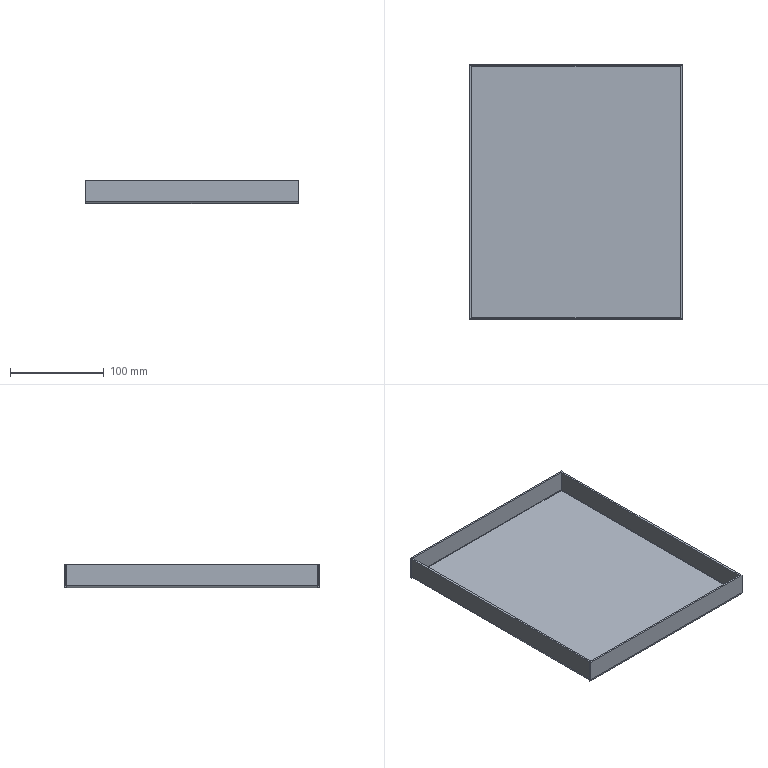Part | STEP file | Rear Base Frame-2 | 1 solid | 34 faces | box 228 x 273 x 25 mm | volume 168843 mm3 | plane 26 | cylinder 8 | commonest cylinder face diameters 1 x4 5 x4
STEP:
#1=CARTESIAN_POINT('',(-827.568,163.879,-2.));
#2=VERTEX_POINT('',#1);
#3=CARTESIAN_POINT('',(-604.568,163.879,-2.));
#4=VERTEX_POINT('',#3);
#5=CARTESIAN_POINT('',(0.,163.879,-2.));
#6=DIRECTION('',(1.,0.,0.));
#7=VECTOR('',#6,1000.);
#8=LINE('',#5,#7);
#9=EDGE_CURVE('',#2,#4,#8,.T.);
#10=ORIENTED_EDGE('',*,*,#9,.T.);
#11=CARTESIAN_POINT('',(-604.568,-104.121,-2.));
#12=VERTEX_POINT('',#11);
#13=CARTESIAN_POINT('',(-604.568,0.,-2.));
#14=DIRECTION('',(0.,-1.,0.));
#15=VECTOR('',#14,1000.);
#16=LINE('',#13,#15);
#17=EDGE_CURVE('',#4,#12,#16,.T.);
#18=ORIENTED_EDGE('',*,*,#17,.T.);
#19=CARTESIAN_POINT('',(-827.568,-104.121,-2.));
#20=VERTEX_POINT('',#19);
#21=CARTESIAN_POINT('',(0.,-104.121,-2.));
#22=DIRECTION('',(-1.,0.,0.));
#23=VECTOR('',#22,1000.);
#24=LINE('',#21,#23);
#25=EDGE_CURVE('',#12,#20,#24,.T.);
#26=ORIENTED_EDGE('',*,*,#25,.T.);
#27=CARTESIAN_POINT('',(-827.568,0.,-2.));
#28=DIRECTION('',(0.,1.,0.));
#29=VECTOR('',#28,1000.);
#30=LINE('',#27,#29);
#31=EDGE_CURVE('',#20,#2,#30,.T.);
#32=ORIENTED_EDGE('',*,*,#31,.T.);
#33=EDGE_LOOP('',(#10,#18,#26,#32));
#34=FACE_OUTER_BOUND('',#33,.T.);
#35=CARTESIAN_POINT('',(0.,0.,-2.));
#36=DIRECTION('',(0.,0.,-1.));
#37=DIRECTION('',(-1.,0.,0.));
#38=AXIS2_PLACEMENT_3D('',#35,#36,#37);
#39=PLANE('',#38);
#40=ADVANCED_FACE('',(#34),#39,.T.);
#41=CARTESIAN_POINT('',(-602.119,-104.121,0.));
#42=VERTEX_POINT('',#41);
#43=CARTESIAN_POINT('',(-602.068,-104.121,0.5));
#44=VERTEX_POINT('',#43);
#45=CARTESIAN_POINT('',(-604.568,-104.121,0.5));
#46=DIRECTION('',(0.,-1.,0.));
#47=DIRECTION('',(0.,0.,1.));
#48=AXIS2_PLACEMENT_3D('',#45,#46,#47);
#49=CIRCLE('',#48,2.5);
#50=EDGE_CURVE('',#42,#44,#49,.T.);
#51=ORIENTED_EDGE('',*,*,#50,.F.);
#52=CARTESIAN_POINT('',(-604.568,-104.121,0.5));
#53=DIRECTION('',(0.,1.,0.));
#54=DIRECTION('',(0.,0.,1.));
#55=AXIS2_PLACEMENT_3D('',#52,#53,#54);
#56=CIRCLE('',#55,2.5);
#57=EDGE_CURVE('',#42,#12,#56,.T.);
#58=ORIENTED_EDGE('',*,*,#57,.T.);
#59=ORIENTED_EDGE('',*,*,#17,.F.);
#60=CARTESIAN_POINT('',(-602.119,163.879,0.));
#61=VERTEX_POINT('',#60);
#62=CARTESIAN_POINT('',(-604.568,163.879,0.5));
#63=DIRECTION('',(0.,-1.,0.));
#64=DIRECTION('',(0.,0.,1.));
#65=AXIS2_PLACEMENT_3D('',#62,#63,#64);
#66=CIRCLE('',#65,2.5);
#67=EDGE_CURVE('',#4,#61,#66,.T.);
#68=ORIENTED_EDGE('',*,*,#67,.T.);
#69=CARTESIAN_POINT('',(-602.068,163.879,0.5));
#70=VERTEX_POINT('',#69);
#71=CARTESIAN_POINT('',(-604.568,163.879,0.5));
#72=DIRECTION('',(0.,-1.,0.));
#73=DIRECTION('',(0.,0.,1.));
#74=AXIS2_PLACEMENT_3D('',#71,#72,#73);
#75=CIRCLE('',#74,2.5);
#76=EDGE_CURVE('',#61,#70,#75,.T.);
#77=ORIENTED_EDGE('',*,*,#76,.T.);
#78=CARTESIAN_POINT('',(-602.068,163.879,0.5));
#79=DIRECTION('',(0.,-1.,0.));
#80=VECTOR('',#79,1000.);
#81=LINE('',#78,#80);
#82=EDGE_CURVE('',#70,#44,#81,.T.);
#83=ORIENTED_EDGE('',*,*,#82,.T.);
#84=EDGE_LOOP('',(#51,#58,#59,#68,#77,#83));
#85=FACE_OUTER_BOUND('',#84,.T.);
#86=CARTESIAN_POINT('',(-604.568,163.879,0.5));
#87=DIRECTION('',(0.,1.,0.));
#88=DIRECTION('',(0.,0.,1.));
#89=AXIS2_PLACEMENT_3D('',#86,#87,#88);
#90=CYLINDRICAL_SURFACE('',#89,2.5);
#91=ADVANCED_FACE('',(#85),#90,.T.);
#92=CARTESIAN_POINT('',(-602.068,163.879,-2.));
#93=VERTEX_POINT('',#92);
#94=CARTESIAN_POINT('',(-830.068,163.879,-2.));
#95=DIRECTION('',(-1.,0.,0.));
#96=VECTOR('',#95,1000.);
#97=LINE('',#94,#96);
#98=EDGE_CURVE('',#93,#4,#97,.T.);
#99=ORIENTED_EDGE('',*,*,#98,.T.);
#100=ORIENTED_EDGE('',*,*,#9,.F.);
#101=CARTESIAN_POINT('',(-830.068,163.879,-2.));
#102=VERTEX_POINT('',#101);
#103=CARTESIAN_POINT('',(-830.068,163.879,-2.));
#104=DIRECTION('',(-1.,0.,0.));
#105=VECTOR('',#104,1000.);
#106=LINE('',#103,#105);
#107=EDGE_CURVE('',#2,#102,#106,.T.);
#108=ORIENTED_EDGE('',*,*,#107,.T.);
#109=CARTESIAN_POINT('',(-830.068,166.379,0.5));
#110=VERTEX_POINT('',#109);
#111=CARTESIAN_POINT('',(-830.068,163.879,0.5));
#112=DIRECTION('',(1.,0.,0.));
#113=DIRECTION('',(0.,0.,1.));
#114=AXIS2_PLACEMENT_3D('',#111,#112,#113);
#115=CIRCLE('',#114,2.5);
#116=EDGE_CURVE('',#102,#110,#115,.T.);
#117=ORIENTED_EDGE('',*,*,#116,.T.);
#118=CARTESIAN_POINT('',(-602.068,166.379,0.5));
#119=VERTEX_POINT('',#118);
#120=CARTESIAN_POINT('',(-830.068,166.379,0.5));
#121=DIRECTION('',(1.,0.,0.));
#122=VECTOR('',#121,1000.);
#123=LINE('',#120,#122);
#124=EDGE_CURVE('',#110,#119,#123,.T.);
#125=ORIENTED_EDGE('',*,*,#124,.T.);
#126=CARTESIAN_POINT('',(-602.068,163.879,0.5));
#127=DIRECTION('',(-1.,0.,0.));
#128=DIRECTION('',(0.,0.,1.));
#129=AXIS2_PLACEMENT_3D('',#126,#127,#128);
#130=CIRCLE('',#129,2.5);
#131=EDGE_CURVE('',#119,#93,#130,.T.);
#132=ORIENTED_EDGE('',*,*,#131,.T.);
#133=EDGE_LOOP('',(#99,#100,#108,#117,#125,#132));
#134=FACE_OUTER_BOUND('',#133,.T.);
#135=CARTESIAN_POINT('',(-830.068,163.879,0.5));
#136=DIRECTION('',(-1.,0.,0.));
#137=DIRECTION('',(0.,0.,1.));
#138=AXIS2_PLACEMENT_3D('',#135,#136,#137);
#139=CYLINDRICAL_SURFACE('',#138,2.5);
#140=ADVANCED_FACE('',(#134),#139,.T.);
#141=CARTESIAN_POINT('',(-830.018,163.879,0.));
#142=VERTEX_POINT('',#141);
#143=CARTESIAN_POINT('',(-830.068,163.879,0.5));
#144=VERTEX_POINT('',#143);
#145=CARTESIAN_POINT('',(-827.568,163.879,0.5));
#146=DIRECTION('',(0.,1.,0.));
#147=DIRECTION('',(0.,0.,-1.));
#148=AXIS2_PLACEMENT_3D('',#145,#146,#147);
#149=CIRCLE('',#148,2.5);
#150=EDGE_CURVE('',#142,#144,#149,.T.);
#151=ORIENTED_EDGE('',*,*,#150,.F.);
#152=CARTESIAN_POINT('',(-827.568,163.879,0.5));
#153=DIRECTION('',(0.,-1.,0.));
#154=DIRECTION('',(0.,0.,-1.));
#155=AXIS2_PLACEMENT_3D('',#152,#153,#154);
#156=CIRCLE('',#155,2.5);
#157=EDGE_CURVE('',#142,#2,#156,.T.);
#158=ORIENTED_EDGE('',*,*,#157,.T.);
#159=ORIENTED_EDGE('',*,*,#31,.F.);
#160=CARTESIAN_POINT('',(-830.018,-104.121,0.));
#161=VERTEX_POINT('',#160);
#162=CARTESIAN_POINT('',(-827.568,-104.121,0.5));
#163=DIRECTION('',(0.,1.,0.));
#164=DIRECTION('',(0.,0.,-1.));
#165=AXIS2_PLACEMENT_3D('',#162,#163,#164);
#166=CIRCLE('',#165,2.5);
#167=EDGE_CURVE('',#20,#161,#166,.T.);
#168=ORIENTED_EDGE('',*,*,#167,.T.);
#169=CARTESIAN_POINT('',(-830.068,-104.121,0.5));
#170=VERTEX_POINT('',#169);
#171=CARTESIAN_POINT('',(-827.568,-104.121,0.5));
#172=DIRECTION('',(0.,1.,0.));
#173=DIRECTION('',(0.,0.,-1.));
#174=AXIS2_PLACEMENT_3D('',#171,#172,#173);
#175=CIRCLE('',#174,2.5);
#176=EDGE_CURVE('',#161,#170,#175,.T.);
#177=ORIENTED_EDGE('',*,*,#176,.T.);
#178=CARTESIAN_POINT('',(-830.068,-104.121,0.5));
#179=DIRECTION('',(0.,1.,0.));
#180=VECTOR('',#179,1000.);
#181=LINE('',#178,#180);
#182=EDGE_CURVE('',#170,#144,#181,.T.);
#183=ORIENTED_EDGE('',*,*,#182,.T.);
#184=EDGE_LOOP('',(#151,#158,#159,#168,#177,#183));
#185=FACE_OUTER_BOUND('',#184,.T.);
#186=CARTESIAN_POINT('',(-827.568,-104.121,0.5));
#187=DIRECTION('',(0.,-1.,0.));
#188=DIRECTION('',(0.,0.,-1.));
#189=AXIS2_PLACEMENT_3D('',#186,#187,#188);
#190=CYLINDRICAL_SURFACE('',#189,2.5);
#191=ADVANCED_FACE('',(#185),#190,.T.);
#192=CARTESIAN_POINT('',(-830.068,-104.121,-2.));
#193=VERTEX_POINT('',#192);
#194=CARTESIAN_POINT('',(-602.068,-104.121,-2.));
#195=DIRECTION('',(1.,0.,0.));
#196=VECTOR('',#195,1000.);
#197=LINE('',#194,#196);
#198=EDGE_CURVE('',#193,#20,#197,.T.);
#199=ORIENTED_EDGE('',*,*,#198,.T.);
#200=ORIENTED_EDGE('',*,*,#25,.F.);
#201=CARTESIAN_POINT('',(-602.068,-104.121,-2.));
#202=VERTEX_POINT('',#201);
#203=CARTESIAN_POINT('',(-602.068,-104.121,-2.));
#204=DIRECTION('',(1.,0.,0.));
#205=VECTOR('',#204,1000.);
#206=LINE('',#203,#205);
#207=EDGE_CURVE('',#12,#202,#206,.T.);
#208=ORIENTED_EDGE('',*,*,#207,.T.);
#209=CARTESIAN_POINT('',(-602.068,-106.621,0.5));
#210=VERTEX_POINT('',#209);
#211=CARTESIAN_POINT('',(-602.068,-104.121,0.5));
#212=DIRECTION('',(-1.,0.,0.));
#213=DIRECTION('',(0.,0.,-1.));
#214=AXIS2_PLACEMENT_3D('',#211,#212,#213);
#215=CIRCLE('',#214,2.5);
#216=EDGE_CURVE('',#202,#210,#215,.T.);
#217=ORIENTED_EDGE('',*,*,#216,.T.);
#218=CARTESIAN_POINT('',(-830.068,-106.621,0.5));
#219=VERTEX_POINT('',#218);
#220=CARTESIAN_POINT('',(-602.068,-106.621,0.5));
#221=DIRECTION('',(-1.,0.,0.));
#222=VECTOR('',#221,1000.);
#223=LINE('',#220,#222);
#224=EDGE_CURVE('',#210,#219,#223,.T.);
#225=ORIENTED_EDGE('',*,*,#224,.T.);
#226=CARTESIAN_POINT('',(-830.068,-104.121,0.5));
#227=DIRECTION('',(1.,0.,0.));
#228=DIRECTION('',(0.,0.,-1.));
#229=AXIS2_PLACEMENT_3D('',#226,#227,#228);
#230=CIRCLE('',#229,2.5);
#231=EDGE_CURVE('',#219,#193,#230,.T.);
#232=ORIENTED_EDGE('',*,*,#231,.T.);
#233=EDGE_LOOP('',(#199,#200,#208,#217,#225,#232));
#234=FACE_OUTER_BOUND('',#233,.T.);
#235=CARTESIAN_POINT('',(-602.068,-104.121,0.5));
#236=DIRECTION('',(1.,0.,0.));
#237=DIRECTION('',(0.,0.,-1.));
#238=AXIS2_PLACEMENT_3D('',#235,#236,#237);
#239=CYLINDRICAL_SURFACE('',#238,2.5);
#240=ADVANCED_FACE('',(#234),#239,.T.);
#241=CARTESIAN_POINT('',(-602.068,-104.121,0.));
#242=VERTEX_POINT('',#241);
#243=CARTESIAN_POINT('',(-602.068,-104.121,0.));
#244=DIRECTION('',(1.,0.,0.));
#245=VECTOR('',#244,1000.);
#246=LINE('',#243,#245);
#247=EDGE_CURVE('',#42,#242,#246,.T.);
#248=ORIENTED_EDGE('',*,*,#247,.T.);
#249=CARTESIAN_POINT('',(-602.068,-104.121,0.));
#250=DIRECTION('',(0.,0.,-1.));
#251=VECTOR('',#250,1000.);
#252=LINE('',#249,#251);
#253=EDGE_CURVE('',#242,#202,#252,.T.);
#254=ORIENTED_EDGE('',*,*,#253,.T.);
#255=ORIENTED_EDGE('',*,*,#207,.F.);
#256=ORIENTED_EDGE('',*,*,#57,.F.);
#257=EDGE_LOOP('',(#248,#254,#255,#256));
#258=FACE_OUTER_BOUND('',#257,.T.);
#259=CARTESIAN_POINT('',(-604.568,-104.121,0.));
#260=DIRECTION('',(0.,1.,0.));
#261=DIRECTION('',(0.,0.,1.));
#262=AXIS2_PLACEMENT_3D('',#259,#260,#261);
#263=PLANE('',#262);
#264=ADVANCED_FACE('',(#258),#263,.T.);
#265=CARTESIAN_POINT('',(-602.068,163.879,23.));
#266=VERTEX_POINT('',#265);
#267=CARTESIAN_POINT('',(-602.068,163.879,0.));
#268=DIRECTION('',(0.,0.,-1.));
#269=VECTOR('',#268,1000.);
#270=LINE('',#267,#269);
#271=EDGE_CURVE('',#266,#70,#270,.T.);
#272=ORIENTED_EDGE('',*,*,#271,.F.);
#273=CARTESIAN_POINT('',(-602.068,-104.121,23.));
#274=VERTEX_POINT('',#273);
#275=CARTESIAN_POINT('',(-602.068,0.,23.));
#276=DIRECTION('',(0.,1.,0.));
#277=VECTOR('',#276,1000.);
#278=LINE('',#275,#277);
#279=EDGE_CURVE('',#274,#266,#278,.T.);
#280=ORIENTED_EDGE('',*,*,#279,.F.);
#281=CARTESIAN_POINT('',(-602.068,-104.121,0.));
#282=DIRECTION('',(0.,0.,1.));
#283=VECTOR('',#282,1000.);
#284=LINE('',#281,#283);
#285=EDGE_CURVE('',#44,#274,#284,.T.);
#286=ORIENTED_EDGE('',*,*,#285,.F.);
#287=ORIENTED_EDGE('',*,*,#82,.F.);
#288=EDGE_LOOP('',(#272,#280,#286,#287));
#289=FACE_OUTER_BOUND('',#288,.T.);
#290=CARTESIAN_POINT('',(-602.068,0.,0.));
#291=DIRECTION('',(-1.,0.,0.));
#292=DIRECTION('',(0.,0.,1.));
#293=AXIS2_PLACEMENT_3D('',#290,#291,#292);
#294=PLANE('',#293);
#295=ADVANCED_FACE('',(#289),#294,.F.);
#296=ORIENTED_EDGE('',*,*,#98,.F.);
#297=CARTESIAN_POINT('',(-602.068,163.879,0.));
#298=VERTEX_POINT('',#297);
#299=CARTESIAN_POINT('',(-602.068,163.879,0.));
#300=DIRECTION('',(0.,0.,1.));
#301=VECTOR('',#300,1000.);
#302=LINE('',#299,#301);
#303=EDGE_CURVE('',#93,#298,#302,.T.);
#304=ORIENTED_EDGE('',*,*,#303,.T.);
#305=CARTESIAN_POINT('',(-830.068,163.879,0.));
#306=DIRECTION('',(-1.,0.,0.));
#307=VECTOR('',#306,1000.);
#308=LINE('',#305,#307);
#309=EDGE_CURVE('',#298,#61,#308,.T.);
#310=ORIENTED_EDGE('',*,*,#309,.T.);
#311=ORIENTED_EDGE('',*,*,#67,.F.);
#312=EDGE_LOOP('',(#296,#304,#310,#311));
#313=FACE_OUTER_BOUND('',#312,.T.);
#314=CARTESIAN_POINT('',(-602.068,163.879,0.));
#315=DIRECTION('',(0.,-1.,0.));
#316=DIRECTION('',(0.,0.,-1.));
#317=AXIS2_PLACEMENT_3D('',#314,#315,#316);
#318=PLANE('',#317);
#319=ADVANCED_FACE('',(#313),#318,.T.);
#320=ORIENTED_EDGE('',*,*,#303,.F.);
#321=ORIENTED_EDGE('',*,*,#131,.F.);
#322=CARTESIAN_POINT('',(-602.068,166.379,23.));
#323=VERTEX_POINT('',#322);
#324=CARTESIAN_POINT('',(-602.068,166.379,0.));
#325=DIRECTION('',(0.,0.,1.));
#326=VECTOR('',#325,1000.);
#327=LINE('',#324,#326);
#328=EDGE_CURVE('',#119,#323,#327,.T.);
#329=ORIENTED_EDGE('',*,*,#328,.T.);
#330=CARTESIAN_POINT('',(-602.068,164.379,23.));
#331=VERTEX_POINT('',#330);
#332=CARTESIAN_POINT('',(-602.068,166.379,23.));
#333=DIRECTION('',(0.,1.,0.));
#334=VECTOR('',#333,1000.);
#335=LINE('',#332,#334);
#336=EDGE_CURVE('',#331,#323,#335,.T.);
#337=ORIENTED_EDGE('',*,*,#336,.F.);
#338=CARTESIAN_POINT('',(-602.068,164.379,0.5));
#339=VERTEX_POINT('',#338);
#340=CARTESIAN_POINT('',(-602.068,164.379,0.));
#341=DIRECTION('',(0.,0.,1.));
#342=VECTOR('',#341,1000.);
#343=LINE('',#340,#342);
#344=EDGE_CURVE('',#339,#331,#343,.T.);
#345=ORIENTED_EDGE('',*,*,#344,.F.);
#346=CARTESIAN_POINT('',(-602.068,163.879,0.5));
#347=DIRECTION('',(-1.,0.,0.));
#348=DIRECTION('',(0.,0.,1.));
#349=AXIS2_PLACEMENT_3D('',#346,#347,#348);
#350=CIRCLE('',#349,0.5);
#351=EDGE_CURVE('',#339,#298,#350,.T.);
#352=ORIENTED_EDGE('',*,*,#351,.T.);
#353=EDGE_LOOP('',(#320,#321,#329,#337,#345,#352));
#354=FACE_OUTER_BOUND('',#353,.T.);
#355=CARTESIAN_POINT('',(-602.068,163.879,0.5));
#356=DIRECTION('',(1.,0.,0.));
#357=DIRECTION('',(0.,0.,-1.));
#358=AXIS2_PLACEMENT_3D('',#355,#356,#357);
#359=PLANE('',#358);
#360=ADVANCED_FACE('',(#354),#359,.T.);
#361=CARTESIAN_POINT('',(-830.068,166.379,23.));
#362=VERTEX_POINT('',#361);
#363=CARTESIAN_POINT('',(-830.068,166.379,0.));
#364=DIRECTION('',(0.,0.,-1.));
#365=VECTOR('',#364,1000.);
#366=LINE('',#363,#365);
#367=EDGE_CURVE('',#362,#110,#366,.T.);
#368=ORIENTED_EDGE('',*,*,#367,.F.);
#369=CARTESIAN_POINT('',(0.,166.379,23.));
#370=DIRECTION('',(-1.,0.,0.));
#371=VECTOR('',#370,1000.);
#372=LINE('',#369,#371);
#373=EDGE_CURVE('',#323,#362,#372,.T.);
#374=ORIENTED_EDGE('',*,*,#373,.F.);
#375=ORIENTED_EDGE('',*,*,#328,.F.);
#376=ORIENTED_EDGE('',*,*,#124,.F.);
#377=EDGE_LOOP('',(#368,#374,#375,#376));
#378=FACE_OUTER_BOUND('',#377,.T.);
#379=CARTESIAN_POINT('',(0.,166.379,0.));
#380=DIRECTION('',(0.,-1.,0.));
#381=DIRECTION('',(0.,0.,-1.));
#382=AXIS2_PLACEMENT_3D('',#379,#380,#381);
#383=PLANE('',#382);
#384=ADVANCED_FACE('',(#378),#383,.F.);
#385=CARTESIAN_POINT('',(-830.068,163.879,0.));
#386=VERTEX_POINT('',#385);
#387=CARTESIAN_POINT('',(-830.068,164.379,0.5));
#388=VERTEX_POINT('',#387);
#389=CARTESIAN_POINT('',(-830.068,163.879,0.5));
#390=DIRECTION('',(1.,0.,0.));
#391=DIRECTION('',(0.,0.,1.));
#392=AXIS2_PLACEMENT_3D('',#389,#390,#391);
#393=CIRCLE('',#392,0.5);
#394=EDGE_CURVE('',#386,#388,#393,.T.);
#395=ORIENTED_EDGE('',*,*,#394,.T.);
#396=CARTESIAN_POINT('',(-830.068,164.379,23.));
#397=VERTEX_POINT('',#396);
#398=CARTESIAN_POINT('',(-830.068,164.379,23.));
#399=DIRECTION('',(0.,0.,-1.));
#400=VECTOR('',#399,1000.);
#401=LINE('',#398,#400);
#402=EDGE_CURVE('',#397,#388,#401,.T.);
#403=ORIENTED_EDGE('',*,*,#402,.F.);
#404=CARTESIAN_POINT('',(-830.068,166.379,23.));
#405=DIRECTION('',(0.,-1.,0.));
#406=VECTOR('',#405,1000.);
#407=LINE('',#404,#406);
#408=EDGE_CURVE('',#362,#397,#407,.T.);
#409=ORIENTED_EDGE('',*,*,#408,.F.);
#410=ORIENTED_EDGE('',*,*,#367,.T.);
#411=ORIENTED_EDGE('',*,*,#116,.F.);
#412=CARTESIAN_POINT('',(-830.068,163.879,0.5));
#413=DIRECTION('',(0.,0.,-1.));
#414=VECTOR('',#413,1000.);
#415=LINE('',#412,#414);
#416=EDGE_CURVE('',#386,#102,#415,.T.);
#417=ORIENTED_EDGE('',*,*,#416,.F.);
#418=EDGE_LOOP('',(#395,#403,#409,#410,#411,#417));
#419=FACE_OUTER_BOUND('',#418,.T.);
#420=CARTESIAN_POINT('',(-830.068,163.879,0.5));
#421=DIRECTION('',(1.,0.,0.));
#422=DIRECTION('',(0.,0.,-1.));
#423=AXIS2_PLACEMENT_3D('',#420,#421,#422);
#424=PLANE('',#423);
#425=ADVANCED_FACE('',(#419),#424,.F.);
#426=CARTESIAN_POINT('',(-830.068,163.879,0.));
#427=DIRECTION('',(-1.,0.,0.));
#428=VECTOR('',#427,1000.);
#429=LINE('',#426,#428);
#430=EDGE_CURVE('',#142,#386,#429,.T.);
#431=ORIENTED_EDGE('',*,*,#430,.T.);
#432=ORIENTED_EDGE('',*,*,#416,.T.);
#433=ORIENTED_EDGE('',*,*,#107,.F.);
#434=ORIENTED_EDGE('',*,*,#157,.F.);
#435=EDGE_LOOP('',(#431,#432,#433,#434));
#436=FACE_OUTER_BOUND('',#435,.T.);
#437=CARTESIAN_POINT('',(-827.568,163.879,0.));
#438=DIRECTION('',(0.,-1.,0.));
#439=DIRECTION('',(0.,0.,-1.));
#440=AXIS2_PLACEMENT_3D('',#437,#438,#439);
#441=PLANE('',#440);
#442=ADVANCED_FACE('',(#436),#441,.T.);
#443=CARTESIAN_POINT('',(-830.068,-104.121,23.));
#444=VERTEX_POINT('',#443);
#445=CARTESIAN_POINT('',(-830.068,-104.121,0.));
#446=DIRECTION('',(0.,0.,-1.));
#447=VECTOR('',#446,1000.);
#448=LINE('',#445,#447);
#449=EDGE_CURVE('',#444,#170,#448,.T.);
#450=ORIENTED_EDGE('',*,*,#449,.F.);
#451=CARTESIAN_POINT('',(-830.068,163.879,23.));
#452=VERTEX_POINT('',#451);
#453=CARTESIAN_POINT('',(-830.068,0.,23.));
#454=DIRECTION('',(0.,-1.,0.));
#455=VECTOR('',#454,1000.);
#456=LINE('',#453,#455);
#457=EDGE_CURVE('',#452,#444,#456,.T.);
#458=ORIENTED_EDGE('',*,*,#457,.F.);
#459=CARTESIAN_POINT('',(-830.068,163.879,0.));
#460=DIRECTION('',(0.,0.,1.));
#461=VECTOR('',#460,1000.);
#462=LINE('',#459,#461);
#463=EDGE_CURVE('',#144,#452,#462,.T.);
#464=ORIENTED_EDGE('',*,*,#463,.F.);
#465=ORIENTED_EDGE('',*,*,#182,.F.);
#466=EDGE_LOOP('',(#450,#458,#464,#465));
#467=FACE_OUTER_BOUND('',#466,.T.);
#468=CARTESIAN_POINT('',(-830.068,0.,0.));
#469=DIRECTION('',(1.,0.,0.));
#470=DIRECTION('',(0.,0.,-1.));
#471=AXIS2_PLACEMENT_3D('',#468,#469,#470);
#472=PLANE('',#471);
#473=ADVANCED_FACE('',(#467),#472,.F.);
#474=ORIENTED_EDGE('',*,*,#198,.F.);
#475=CARTESIAN_POINT('',(-830.068,-104.121,0.));
#476=VERTEX_POINT('',#475);
#477=CARTESIAN_POINT('',(-830.068,-104.121,0.));
#478=DIRECTION('',(0.,0.,1.));
#479=VECTOR('',#478,1000.);
#480=LINE('',#477,#479);
#481=EDGE_CURVE('',#193,#476,#480,.T.);
#482=ORIENTED_EDGE('',*,*,#481,.T.);
#483=CARTESIAN_POINT('',(-602.068,-104.121,0.));
#484=DIRECTION('',(1.,0.,0.));
#485=VECTOR('',#484,1000.);
#486=LINE('',#483,#485);
#487=EDGE_CURVE('',#476,#161,#486,.T.);
#488=ORIENTED_EDGE('',*,*,#487,.T.);
#489=ORIENTED_EDGE('',*,*,#167,.F.);
#490=EDGE_LOOP('',(#474,#482,#488,#489));
#491=FACE_OUTER_BOUND('',#490,.T.);
#492=CARTESIAN_POINT('',(-830.068,-104.121,0.));
#493=DIRECTION('',(0.,1.,0.));
#494=DIRECTION('',(-1.,0.,0.));
#495=AXIS2_PLACEMENT_3D('',#492,#493,#494);
#496=PLANE('',#495);
#497=ADVANCED_FACE('',(#491),#496,.T.);
#498=ORIENTED_EDGE('',*,*,#481,.F.);
#499=ORIENTED_EDGE('',*,*,#231,.F.);
#500=CARTESIAN_POINT('',(-830.068,-106.621,23.));
#501=VERTEX_POINT('',#500);
#502=CARTESIAN_POINT('',(-830.068,-106.621,0.));
#503=DIRECTION('',(0.,0.,1.));
#504=VECTOR('',#503,1000.);
#505=LINE('',#502,#504);
#506=EDGE_CURVE('',#219,#501,#505,.T.);
#507=ORIENTED_EDGE('',*,*,#506,.T.);
#508=CARTESIAN_POINT('',(-830.068,-104.621,23.));
#509=VERTEX_POINT('',#508);
#510=CARTESIAN_POINT('',(-830.068,-106.621,23.));
#511=DIRECTION('',(0.,-1.,0.));
#512=VECTOR('',#511,1000.);
#513=LINE('',#510,#512);
#514=EDGE_CURVE('',#509,#501,#513,.T.);
#515=ORIENTED_EDGE('',*,*,#514,.F.);
#516=CARTESIAN_POINT('',(-830.068,-104.621,0.5));
#517=VERTEX_POINT('',#516);
#518=CARTESIAN_POINT('',(-830.068,-104.621,0.));
#519=DIRECTION('',(0.,0.,1.));
#520=VECTOR('',#519,1000.);
#521=LINE('',#518,#520);
#522=EDGE_CURVE('',#517,#509,#521,.T.);
#523=ORIENTED_EDGE('',*,*,#522,.F.);
#524=CARTESIAN_POINT('',(-830.068,-104.121,0.5));
#525=DIRECTION('',(1.,0.,0.));
#526=DIRECTION('',(0.,0.,-1.));
#527=AXIS2_PLACEMENT_3D('',#524,#525,#526);
#528=CIRCLE('',#527,0.5);
#529=EDGE_CURVE('',#517,#476,#528,.T.);
#530=ORIENTED_EDGE('',*,*,#529,.T.);
#531=EDGE_LOOP('',(#498,#499,#507,#515,#523,#530));
#532=FACE_OUTER_BOUND('',#531,.T.);
#533=CARTESIAN_POINT('',(-830.068,-104.121,0.5));
#534=DIRECTION('',(-1.,0.,0.));
#535=DIRECTION('',(0.,0.,1.));
#536=AXIS2_PLACEMENT_3D('',#533,#534,#535);
#537=PLANE('',#536);
#538=ADVANCED_FACE('',(#532),#537,.T.);
#539=CARTESIAN_POINT('',(-602.068,-106.621,23.));
#540=VERTEX_POINT('',#539);
#541=CARTESIAN_POINT('',(-602.068,-106.621,0.));
#542=DIRECTION('',(0.,0.,-1.));
#543=VECTOR('',#542,1000.);
#544=LINE('',#541,#543);
#545=EDGE_CURVE('',#540,#210,#544,.T.);
#546=ORIENTED_EDGE('',*,*,#545,.F.);
#547=CARTESIAN_POINT('',(0.,-106.621,23.));
#548=DIRECTION('',(1.,0.,0.));
#549=VECTOR('',#548,1000.);
#550=LINE('',#547,#549);
#551=EDGE_CURVE('',#501,#540,#550,.T.);
#552=ORIENTED_EDGE('',*,*,#551,.F.);
#553=ORIENTED_EDGE('',*,*,#506,.F.);
#554=ORIENTED_EDGE('',*,*,#224,.F.);
#555=EDGE_LOOP('',(#546,#552,#553,#554));
#556=FACE_OUTER_BOUND('',#555,.T.);
#557=CARTESIAN_POINT('',(0.,-106.621,0.));
#558=DIRECTION('',(0.,1.,0.));
#559=DIRECTION('',(0.,0.,1.));
#560=AXIS2_PLACEMENT_3D('',#557,#558,#559);
#561=PLANE('',#560);
#562=ADVANCED_FACE('',(#556),#561,.F.);
#563=CARTESIAN_POINT('',(-602.068,-104.621,0.5));
#564=VERTEX_POINT('',#563);
#565=CARTESIAN_POINT('',(-602.068,-104.121,0.5));
#566=DIRECTION('',(-1.,0.,0.));
#567=DIRECTION('',(0.,0.,-1.));
#568=AXIS2_PLACEMENT_3D('',#565,#566,#567);
#569=CIRCLE('',#568,0.5);
#570=EDGE_CURVE('',#242,#564,#569,.T.);
#571=ORIENTED_EDGE('',*,*,#570,.T.);
#572=CARTESIAN_POINT('',(-602.068,-104.621,23.));
#573=VERTEX_POINT('',#572);
#574=CARTESIAN_POINT('',(-602.068,-104.621,23.));
#575=DIRECTION('',(0.,0.,-1.));
#576=VECTOR('',#575,1000.);
#577=LINE('',#574,#576);
#578=EDGE_CURVE('',#573,#564,#577,.T.);
#579=ORIENTED_EDGE('',*,*,#578,.F.);
#580=CARTESIAN_POINT('',(-602.068,-106.621,23.));
#581=DIRECTION('',(0.,1.,0.));
#582=VECTOR('',#581,1000.);
#583=LINE('',#580,#582);
#584=EDGE_CURVE('',#540,#573,#583,.T.);
#585=ORIENTED_EDGE('',*,*,#584,.F.);
#586=ORIENTED_EDGE('',*,*,#545,.T.);
#587=ORIENTED_EDGE('',*,*,#216,.F.);
#588=ORIENTED_EDGE('',*,*,#253,.F.);
#589=EDGE_LOOP('',(#571,#579,#585,#586,#587,#588));
#590=FACE_OUTER_BOUND('',#589,.T.);
#591=CARTESIAN_POINT('',(-602.068,-104.121,0.5));
#592=DIRECTION('',(-1.,0.,0.));
#593=DIRECTION('',(0.,0.,1.));
#594=AXIS2_PLACEMENT_3D('',#591,#592,#593);
#595=PLANE('',#594);
#596=ADVANCED_FACE('',(#590),#595,.F.);
#597=CARTESIAN_POINT('',(-604.068,163.879,23.));
#598=VERTEX_POINT('',#597);
#599=CARTESIAN_POINT('',(-604.068,163.879,0.5));
#600=VERTEX_POINT('',#599);
#601=CARTESIAN_POINT('',(-604.068,163.879,23.));
#602=DIRECTION('',(0.,0.,-1.));
#603=VECTOR('',#602,1000.);
#604=LINE('',#601,#603);
#605=EDGE_CURVE('',#598,#600,#604,.T.);
#606=ORIENTED_EDGE('',*,*,#605,.F.);
#607=CARTESIAN_POINT('',(-602.068,163.879,23.));
#608=DIRECTION('',(-1.,0.,0.));
#609=VECTOR('',#608,1000.);
#610=LINE('',#607,#609);
#611=EDGE_CURVE('',#266,#598,#610,.T.);
#612=ORIENTED_EDGE('',*,*,#611,.F.);
#613=ORIENTED_EDGE('',*,*,#271,.T.);
#614=ORIENTED_EDGE('',*,*,#76,.F.);
#615=CARTESIAN_POINT('',(-604.568,163.879,0.));
#616=VERTEX_POINT('',#615);
#617=CARTESIAN_POINT('',(-604.568,163.879,0.));
#618=DIRECTION('',(1.,0.,0.));
#619=VECTOR('',#618,1000.);
#620=LINE('',#617,#619);
#621=EDGE_CURVE('',#616,#61,#620,.T.);
#622=ORIENTED_EDGE('',*,*,#621,.F.);
#623=CARTESIAN_POINT('',(-604.568,163.879,0.5));
#624=DIRECTION('',(0.,-1.,0.));
#625=DIRECTION('',(0.,0.,1.));
#626=AXIS2_PLACEMENT_3D('',#623,#624,#625);
#627=CIRCLE('',#626,0.5);
#628=EDGE_CURVE('',#616,#600,#627,.T.);
#629=ORIENTED_EDGE('',*,*,#628,.T.);
#630=EDGE_LOOP('',(#606,#612,#613,#614,#622,#629));
#631=FACE_OUTER_BOUND('',#630,.T.);
#632=CARTESIAN_POINT('',(-602.068,163.879,23.));
#633=DIRECTION('',(0.,-1.,0.));
#634=DIRECTION('',(1.,0.,0.));
#635=AXIS2_PLACEMENT_3D('',#632,#633,#634);
#636=PLANE('',#635);
#637=ADVANCED_FACE('',(#631),#636,.F.);
#638=CARTESIAN_POINT('',(-604.068,-104.121,23.));
#639=VERTEX_POINT('',#638);
#640=CARTESIAN_POINT('',(-602.068,-104.121,23.));
#641=DIRECTION('',(-1.,0.,0.));
#642=VECTOR('',#641,1000.);
#643=LINE('',#640,#642);
#644=EDGE_CURVE('',#274,#639,#643,.T.);
#645=ORIENTED_EDGE('',*,*,#644,.F.);
#646=ORIENTED_EDGE('',*,*,#279,.T.);
#647=ORIENTED_EDGE('',*,*,#611,.T.);
#648=CARTESIAN_POINT('',(-604.068,-104.121,23.));
#649=DIRECTION('',(0.,1.,0.));
#650=VECTOR('',#649,1000.);
#651=LINE('',#648,#650);
#652=EDGE_CURVE('',#639,#598,#651,.T.);
#653=ORIENTED_EDGE('',*,*,#652,.F.);
#654=EDGE_LOOP('',(#645,#646,#647,#653));
#655=FACE_OUTER_BOUND('',#654,.T.);
#656=CARTESIAN_POINT('',(-602.068,-104.121,23.));
#657=DIRECTION('',(0.,0.,-1.));
#658=DIRECTION('',(-1.,0.,0.));
#659=AXIS2_PLACEMENT_3D('',#656,#657,#658);
#660=PLANE('',#659);
#661=ADVANCED_FACE('',(#655),#660,.F.);
#662=ORIENTED_EDGE('',*,*,#285,.T.);
#663=ORIENTED_EDGE('',*,*,#644,.T.);
#664=CARTESIAN_POINT('',(-604.068,-104.121,0.5));
#665=VERTEX_POINT('',#664);
#666=CARTESIAN_POINT('',(-604.068,-104.121,0.));
#667=DIRECTION('',(0.,0.,1.));
#668=VECTOR('',#667,1000.);
#669=LINE('',#666,#668);
#670=EDGE_CURVE('',#665,#639,#669,.T.);
#671=ORIENTED_EDGE('',*,*,#670,.F.);
#672=CARTESIAN_POINT('',(-604.568,-104.121,0.));
#673=VERTEX_POINT('',#672);
#674=CARTESIAN_POINT('',(-604.568,-104.121,0.5));
#675=DIRECTION('',(0.,1.,0.));
#676=DIRECTION('',(0.,0.,1.));
#677=AXIS2_PLACEMENT_3D('',#674,#675,#676);
#678=CIRCLE('',#677,0.5);
#679=EDGE_CURVE('',#665,#673,#678,.T.);
#680=ORIENTED_EDGE('',*,*,#679,.T.);
#681=CARTESIAN_POINT('',(-604.568,-104.121,0.));
#682=DIRECTION('',(1.,0.,0.));
#683=VECTOR('',#682,1000.);
#684=LINE('',#681,#683);
#685=EDGE_CURVE('',#673,#42,#684,.T.);
#686=ORIENTED_EDGE('',*,*,#685,.T.);
#687=ORIENTED_EDGE('',*,*,#50,.T.);
#688=EDGE_LOOP('',(#662,#663,#671,#680,#686,#687));
#689=FACE_OUTER_BOUND('',#688,.T.);
#690=CARTESIAN_POINT('',(-602.068,-104.121,0.));
#691=DIRECTION('',(0.,1.,0.));
#692=DIRECTION('',(-1.,0.,0.));
#693=AXIS2_PLACEMENT_3D('',#690,#691,#692);
#694=PLANE('',#693);
#695=ADVANCED_FACE('',(#689),#694,.F.);
#696=ORIENTED_EDGE('',*,*,#336,.T.);
#697=ORIENTED_EDGE('',*,*,#373,.T.);
#698=ORIENTED_EDGE('',*,*,#408,.T.);
#699=CARTESIAN_POINT('',(-602.068,164.379,23.));
#700=DIRECTION('',(-1.,0.,0.));
#701=VECTOR('',#700,1000.);
#702=LINE('',#699,#701);
#703=EDGE_CURVE('',#331,#397,#702,.T.);
#704=ORIENTED_EDGE('',*,*,#703,.F.);
#705=EDGE_LOOP('',(#696,#697,#698,#704));
#706=FACE_OUTER_BOUND('',#705,.T.);
#707=CARTESIAN_POINT('',(-602.068,166.379,23.));
#708=DIRECTION('',(0.,0.,-1.));
#709=DIRECTION('',(0.,1.,0.));
#710=AXIS2_PLACEMENT_3D('',#707,#708,#709);
#711=PLANE('',#710);
#712=ADVANCED_FACE('',(#706),#711,.F.);
#713=CARTESIAN_POINT('',(-828.068,-104.121,23.));
#714=VERTEX_POINT('',#713);
#715=CARTESIAN_POINT('',(-828.068,-104.121,0.5));
#716=VERTEX_POINT('',#715);
#717=CARTESIAN_POINT('',(-828.068,-104.121,23.));
#718=DIRECTION('',(0.,0.,-1.));
#719=VECTOR('',#718,1000.);
#720=LINE('',#717,#719);
#721=EDGE_CURVE('',#714,#716,#720,.T.);
#722=ORIENTED_EDGE('',*,*,#721,.F.);
#723=CARTESIAN_POINT('',(-830.068,-104.121,23.));
#724=DIRECTION('',(1.,0.,0.));
#725=VECTOR('',#724,1000.);
#726=LINE('',#723,#725);
#727=EDGE_CURVE('',#444,#714,#726,.T.);
#728=ORIENTED_EDGE('',*,*,#727,.F.);
#729=ORIENTED_EDGE('',*,*,#449,.T.);
#730=ORIENTED_EDGE('',*,*,#176,.F.);
#731=CARTESIAN_POINT('',(-827.568,-104.121,0.));
#732=VERTEX_POINT('',#731);
#733=CARTESIAN_POINT('',(-827.568,-104.121,0.));
#734=DIRECTION('',(-1.,0.,0.));
#735=VECTOR('',#734,1000.);
#736=LINE('',#733,#735);
#737=EDGE_CURVE('',#732,#161,#736,.T.);
#738=ORIENTED_EDGE('',*,*,#737,.F.);
#739=CARTESIAN_POINT('',(-827.568,-104.121,0.5));
#740=DIRECTION('',(0.,1.,0.));
#741=DIRECTION('',(0.,0.,-1.));
#742=AXIS2_PLACEMENT_3D('',#739,#740,#741);
#743=CIRCLE('',#742,0.5);
#744=EDGE_CURVE('',#732,#716,#743,.T.);
#745=ORIENTED_EDGE('',*,*,#744,.T.);
#746=EDGE_LOOP('',(#722,#728,#729,#730,#738,#745));
#747=FACE_OUTER_BOUND('',#746,.T.);
#748=CARTESIAN_POINT('',(-830.068,-104.121,23.));
#749=DIRECTION('',(0.,1.,0.));
#750=DIRECTION('',(0.,0.,1.));
#751=AXIS2_PLACEMENT_3D('',#748,#749,#750);
#752=PLANE('',#751);
#753=ADVANCED_FACE('',(#747),#752,.F.);
#754=CARTESIAN_POINT('',(-828.068,163.879,23.));
#755=VERTEX_POINT('',#754);
#756=CARTESIAN_POINT('',(-830.068,163.879,23.));
#757=DIRECTION('',(1.,0.,0.));
#758=VECTOR('',#757,1000.);
#759=LINE('',#756,#758);
#760=EDGE_CURVE('',#452,#755,#759,.T.);
#761=ORIENTED_EDGE('',*,*,#760,.F.);
#762=ORIENTED_EDGE('',*,*,#457,.T.);
#763=ORIENTED_EDGE('',*,*,#727,.T.);
#764=CARTESIAN_POINT('',(-828.068,163.879,23.));
#765=DIRECTION('',(0.,-1.,0.));
#766=VECTOR('',#765,1000.);
#767=LINE('',#764,#766);
#768=EDGE_CURVE('',#755,#714,#767,.T.);
#769=ORIENTED_EDGE('',*,*,#768,.F.);
#770=EDGE_LOOP('',(#761,#762,#763,#769));
#771=FACE_OUTER_BOUND('',#770,.T.);
#772=CARTESIAN_POINT('',(-830.068,163.879,23.));
#773=DIRECTION('',(0.,0.,-1.));
#774=DIRECTION('',(-1.,0.,0.));
#775=AXIS2_PLACEMENT_3D('',#772,#773,#774);
#776=PLANE('',#775);
#777=ADVANCED_FACE('',(#771),#776,.F.);
#778=ORIENTED_EDGE('',*,*,#463,.T.);
#779=ORIENTED_EDGE('',*,*,#760,.T.);
#780=CARTESIAN_POINT('',(-828.068,163.879,0.5));
#781=VERTEX_POINT('',#780);
#782=CARTESIAN_POINT('',(-828.068,163.879,0.));
#783=DIRECTION('',(0.,0.,1.));
#784=VECTOR('',#783,1000.);
#785=LINE('',#782,#784);
#786=EDGE_CURVE('',#781,#755,#785,.T.);
#787=ORIENTED_EDGE('',*,*,#786,.F.);
#788=CARTESIAN_POINT('',(-827.568,163.879,0.));
#789=VERTEX_POINT('',#788);
#790=CARTESIAN_POINT('',(-827.568,163.879,0.5));
#791=DIRECTION('',(0.,-1.,0.));
#792=DIRECTION('',(0.,0.,-1.));
#793=AXIS2_PLACEMENT_3D('',#790,#791,#792);
#794=CIRCLE('',#793,0.5);
#795=EDGE_CURVE('',#781,#789,#794,.T.);
#796=ORIENTED_EDGE('',*,*,#795,.T.);
#797=CARTESIAN_POINT('',(-827.568,163.879,0.));
#798=DIRECTION('',(-1.,0.,0.));
#799=VECTOR('',#798,1000.);
#800=LINE('',#797,#799);
#801=EDGE_CURVE('',#789,#142,#800,.T.);
#802=ORIENTED_EDGE('',*,*,#801,.T.);
#803=ORIENTED_EDGE('',*,*,#150,.T.);
#804=EDGE_LOOP('',(#778,#779,#787,#796,#802,#803));
#805=FACE_OUTER_BOUND('',#804,.T.);
#806=CARTESIAN_POINT('',(-830.068,163.879,0.));
#807=DIRECTION('',(0.,-1.,0.));
#808=DIRECTION('',(0.,0.,-1.));
#809=AXIS2_PLACEMENT_3D('',#806,#807,#808);
#810=PLANE('',#809);
#811=ADVANCED_FACE('',(#805),#810,.F.);
#812=ORIENTED_EDGE('',*,*,#514,.T.);
#813=ORIENTED_EDGE('',*,*,#551,.T.);
#814=ORIENTED_EDGE('',*,*,#584,.T.);
#815=CARTESIAN_POINT('',(-830.068,-104.621,23.));
#816=DIRECTION('',(1.,0.,0.));
#817=VECTOR('',#816,1000.);
#818=LINE('',#815,#817);
#819=EDGE_CURVE('',#509,#573,#818,.T.);
#820=ORIENTED_EDGE('',*,*,#819,.F.);
#821=EDGE_LOOP('',(#812,#813,#814,#820));
#822=FACE_OUTER_BOUND('',#821,.T.);
#823=CARTESIAN_POINT('',(-830.068,-106.621,23.));
#824=DIRECTION('',(0.,0.,-1.));
#825=DIRECTION('',(0.,1.,0.));
#826=AXIS2_PLACEMENT_3D('',#823,#824,#825);
#827=PLANE('',#826);
#828=ADVANCED_FACE('',(#822),#827,.F.);
#829=ORIENTED_EDGE('',*,*,#670,.T.);
#830=ORIENTED_EDGE('',*,*,#652,.T.);
#831=ORIENTED_EDGE('',*,*,#605,.T.);
#832=CARTESIAN_POINT('',(-604.068,0.,0.5));
#833=DIRECTION('',(0.,-1.,0.));
#834=VECTOR('',#833,1000.);
#835=LINE('',#832,#834);
#836=EDGE_CURVE('',#600,#665,#835,.T.);
#837=ORIENTED_EDGE('',*,*,#836,.T.);
#838=EDGE_LOOP('',(#829,#830,#831,#837));
#839=FACE_OUTER_BOUND('',#838,.T.);
#840=CARTESIAN_POINT('',(-604.068,0.,0.));
#841=DIRECTION('',(-1.,0.,0.));
#842=DIRECTION('',(0.,0.,1.));
#843=AXIS2_PLACEMENT_3D('',#840,#841,#842);
#844=PLANE('',#843);
#845=ADVANCED_FACE('',(#839),#844,.T.);
#846=ORIENTED_EDGE('',*,*,#344,.T.);
#847=ORIENTED_EDGE('',*,*,#703,.T.);
#848=ORIENTED_EDGE('',*,*,#402,.T.);
#849=CARTESIAN_POINT('',(0.,164.379,0.5));
#850=DIRECTION('',(1.,0.,0.));
#851=VECTOR('',#850,1000.);
#852=LINE('',#849,#851);
#853=EDGE_CURVE('',#388,#339,#852,.T.);
#854=ORIENTED_EDGE('',*,*,#853,.T.);
#855=EDGE_LOOP('',(#846,#847,#848,#854));
#856=FACE_OUTER_BOUND('',#855,.T.);
#857=CARTESIAN_POINT('',(0.,164.379,0.));
#858=DIRECTION('',(0.,-1.,0.));
#859=DIRECTION('',(0.,0.,-1.));
#860=AXIS2_PLACEMENT_3D('',#857,#858,#859);
#861=PLANE('',#860);
#862=ADVANCED_FACE('',(#856),#861,.T.);
#863=ORIENTED_EDGE('',*,*,#786,.T.);
#864=ORIENTED_EDGE('',*,*,#768,.T.);
#865=ORIENTED_EDGE('',*,*,#721,.T.);
#866=CARTESIAN_POINT('',(-828.068,0.,0.5));
#867=DIRECTION('',(0.,1.,0.));
#868=VECTOR('',#867,1000.);
#869=LINE('',#866,#868);
#870=EDGE_CURVE('',#716,#781,#869,.T.);
#871=ORIENTED_EDGE('',*,*,#870,.T.);
#872=EDGE_LOOP('',(#863,#864,#865,#871));
#873=FACE_OUTER_BOUND('',#872,.T.);
#874=CARTESIAN_POINT('',(-828.068,0.,0.));
#875=DIRECTION('',(1.,0.,0.));
#876=DIRECTION('',(0.,0.,-1.));
#877=AXIS2_PLACEMENT_3D('',#874,#875,#876);
#878=PLANE('',#877);
#879=ADVANCED_FACE('',(#873),#878,.T.);
#880=ORIENTED_EDGE('',*,*,#522,.T.);
#881=ORIENTED_EDGE('',*,*,#819,.T.);
#882=ORIENTED_EDGE('',*,*,#578,.T.);
#883=CARTESIAN_POINT('',(0.,-104.621,0.5));
#884=DIRECTION('',(-1.,0.,0.));
#885=VECTOR('',#884,1000.);
#886=LINE('',#883,#885);
#887=EDGE_CURVE('',#564,#517,#886,.T.);
#888=ORIENTED_EDGE('',*,*,#887,.T.);
#889=EDGE_LOOP('',(#880,#881,#882,#888));
#890=FACE_OUTER_BOUND('',#889,.T.);
#891=CARTESIAN_POINT('',(0.,-104.621,0.));
#892=DIRECTION('',(0.,1.,0.));
#893=DIRECTION('',(0.,0.,1.));
#894=AXIS2_PLACEMENT_3D('',#891,#892,#893);
#895=PLANE('',#894);
#896=ADVANCED_FACE('',(#890),#895,.T.);
#897=ORIENTED_EDGE('',*,*,#801,.F.);
#898=CARTESIAN_POINT('',(-830.068,163.879,0.));
#899=DIRECTION('',(-1.,0.,0.));
#900=VECTOR('',#899,1000.);
#901=LINE('',#898,#900);
#902=EDGE_CURVE('',#616,#789,#901,.T.);
#903=ORIENTED_EDGE('',*,*,#902,.F.);
#904=ORIENTED_EDGE('',*,*,#621,.T.);
#905=ORIENTED_EDGE('',*,*,#309,.F.);
#906=ORIENTED_EDGE('',*,*,#351,.F.);
#907=ORIENTED_EDGE('',*,*,#853,.F.);
#908=ORIENTED_EDGE('',*,*,#394,.F.);
#909=ORIENTED_EDGE('',*,*,#430,.F.);
#910=EDGE_LOOP('',(#897,#903,#904,#905,#906,#907,#908,#909));
#911=FACE_OUTER_BOUND('',#910,.T.);
#912=CARTESIAN_POINT('',(-830.068,163.879,0.5));
#913=DIRECTION('',(-1.,0.,0.));
#914=DIRECTION('',(0.,0.,1.));
#915=AXIS2_PLACEMENT_3D('',#912,#913,#914);
#916=CYLINDRICAL_SURFACE('',#915,0.5);
#917=ADVANCED_FACE('',(#911),#916,.F.);
#918=ORIENTED_EDGE('',*,*,#679,.F.);
#919=ORIENTED_EDGE('',*,*,#836,.F.);
#920=ORIENTED_EDGE('',*,*,#628,.F.);
#921=CARTESIAN_POINT('',(-604.568,163.879,0.));
#922=DIRECTION('',(0.,1.,0.));
#923=VECTOR('',#922,1000.);
#924=LINE('',#921,#923);
#925=EDGE_CURVE('',#673,#616,#924,.T.);
#926=ORIENTED_EDGE('',*,*,#925,.F.);
#927=EDGE_LOOP('',(#918,#919,#920,#926));
#928=FACE_OUTER_BOUND('',#927,.T.);
#929=CARTESIAN_POINT('',(-604.568,163.879,0.5));
#930=DIRECTION('',(0.,1.,0.));
#931=DIRECTION('',(0.,0.,1.));
#932=AXIS2_PLACEMENT_3D('',#929,#930,#931);
#933=CYLINDRICAL_SURFACE('',#932,0.5);
#934=ADVANCED_FACE('',(#928),#933,.F.);
#935=ORIENTED_EDGE('',*,*,#685,.F.);
#936=CARTESIAN_POINT('',(-602.068,-104.121,0.));
#937=DIRECTION('',(1.,0.,0.));
#938=VECTOR('',#937,1000.);
#939=LINE('',#936,#938);
#940=EDGE_CURVE('',#732,#673,#939,.T.);
#941=ORIENTED_EDGE('',*,*,#940,.F.);
#942=ORIENTED_EDGE('',*,*,#737,.T.);
#943=ORIENTED_EDGE('',*,*,#487,.F.);
#944=ORIENTED_EDGE('',*,*,#529,.F.);
#945=ORIENTED_EDGE('',*,*,#887,.F.);
#946=ORIENTED_EDGE('',*,*,#570,.F.);
#947=ORIENTED_EDGE('',*,*,#247,.F.);
#948=EDGE_LOOP('',(#935,#941,#942,#943,#944,#945,#946,#947));
#949=FACE_OUTER_BOUND('',#948,.T.);
#950=CARTESIAN_POINT('',(-602.068,-104.121,0.5));
#951=DIRECTION('',(1.,0.,0.));
#952=DIRECTION('',(0.,0.,-1.));
#953=AXIS2_PLACEMENT_3D('',#950,#951,#952);
#954=CYLINDRICAL_SURFACE('',#953,0.5);
#955=ADVANCED_FACE('',(#949),#954,.F.);
#956=ORIENTED_EDGE('',*,*,#795,.F.);
#957=ORIENTED_EDGE('',*,*,#870,.F.);
#958=ORIENTED_EDGE('',*,*,#744,.F.);
#959=CARTESIAN_POINT('',(-827.568,-104.121,0.));
#960=DIRECTION('',(0.,-1.,0.));
#961=VECTOR('',#960,1000.);
#962=LINE('',#959,#961);
#963=EDGE_CURVE('',#789,#732,#962,.T.);
#964=ORIENTED_EDGE('',*,*,#963,.F.);
#965=EDGE_LOOP('',(#956,#957,#958,#964));
#966=FACE_OUTER_BOUND('',#965,.T.);
#967=CARTESIAN_POINT('',(-827.568,-104.121,0.5));
#968=DIRECTION('',(0.,-1.,0.));
#969=DIRECTION('',(0.,0.,-1.));
#970=AXIS2_PLACEMENT_3D('',#967,#968,#969);
#971=CYLINDRICAL_SURFACE('',#970,0.5);
#972=ADVANCED_FACE('',(#966),#971,.F.);
#973=ORIENTED_EDGE('',*,*,#940,.T.);
#974=ORIENTED_EDGE('',*,*,#925,.T.);
#975=ORIENTED_EDGE('',*,*,#902,.T.);
#976=ORIENTED_EDGE('',*,*,#963,.T.);
#977=EDGE_LOOP('',(#973,#974,#975,#976));
#978=FACE_OUTER_BOUND('',#977,.T.);
#979=CARTESIAN_POINT('',(0.,0.,0.));
#980=DIRECTION('',(0.,0.,-1.));
#981=DIRECTION('',(-1.,0.,0.));
#982=AXIS2_PLACEMENT_3D('',#979,#980,#981);
#983=PLANE('',#982);
#984=ADVANCED_FACE('',(#978),#983,.F.);
#985=CLOSED_SHELL('',(#40,#91,#140,#191,#240,#264,#295,#319,#360,#384,#425,#442,#473,#497,#538,#562,#596,#637,#661,#695,#712,#753,#777,#811,#828,#845,#862,#879,#896,#917,#934,#955,#972,#984));
#986=MANIFOLD_SOLID_BREP('',#985);
#987=CARTESIAN_POINT('',(0.,0.,0.));
#988=DIRECTION('',(0.,0.,1.));
#989=DIRECTION('',(1.,0.,0.));
#990=AXIS2_PLACEMENT_3D('',#987,#988,#989);
#991=(LENGTH_UNIT()NAMED_UNIT(*)SI_UNIT(.MILLI.,.METRE.));
#992=UNCERTAINTY_MEASURE_WITH_UNIT(LENGTH_MEASURE(0.00001),#991,'','');
#993=(NAMED_UNIT(*)PLANE_ANGLE_UNIT()SI_UNIT($,.RADIAN.));
#994=(NAMED_UNIT(*)SI_UNIT($,.STERADIAN.)SOLID_ANGLE_UNIT());
#995=(GEOMETRIC_REPRESENTATION_CONTEXT(3)GLOBAL_UNCERTAINTY_ASSIGNED_CONTEXT((#992))GLOBAL_UNIT_ASSIGNED_CONTEXT((#991,#993,#994))REPRESENTATION_CONTEXT('',''));
#996=ADVANCED_BREP_SHAPE_REPRESENTATION('',(#986,#990),#995);